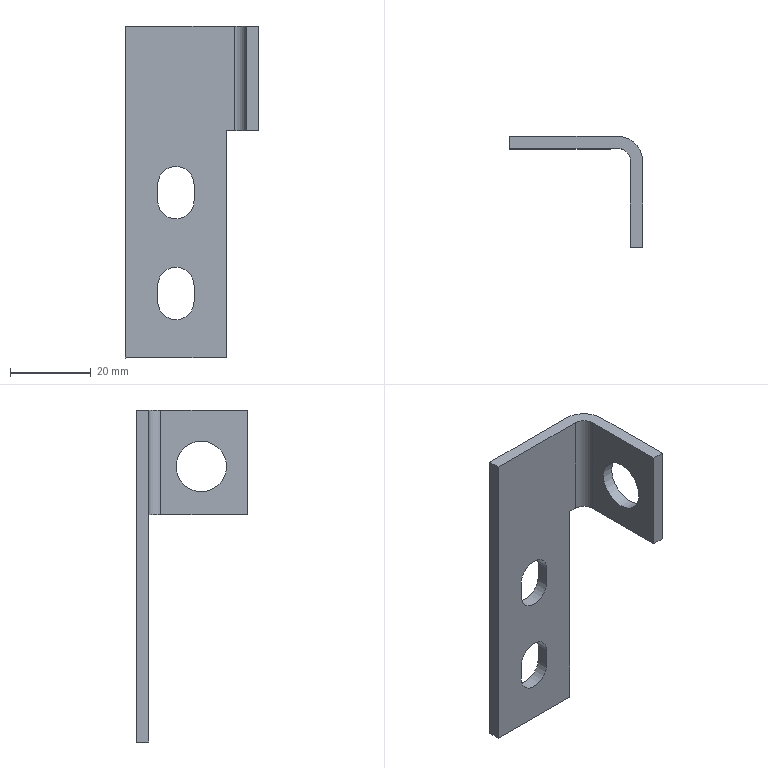Part | STEP file | lll_id850_x_t | 1 solid | 21 faces | box 33 x 27.5 x 82.328 mm | volume 7593 mm3 | plane 14 | cylinder 7 | commonest cylinder face diameters 9 x4 6 x1 12 x1 12.5 x1
STEP:
#1=CARTESIAN_POINT('',(3966.707,-571.677,70.922));
#2=VERTEX_POINT('',#1);
#3=CARTESIAN_POINT('',(3966.707,-571.677,153.25));
#4=VERTEX_POINT('',#3);
#5=CARTESIAN_POINT('',(3966.707,-571.677,181.75));
#6=DIRECTION('',(0.,0.,1.));
#7=VECTOR('',#6,1.);
#8=LINE('',#5,#7);
#9=EDGE_CURVE('',#2,#4,#8,.T.);
#10=ORIENTED_EDGE('',*,*,#9,.F.);
#11=CARTESIAN_POINT('',(3991.707,-571.677,70.922));
#12=VERTEX_POINT('',#11);
#13=CARTESIAN_POINT('',(4574.571,-571.677,70.922));
#14=DIRECTION('',(1.,0.,0.));
#15=VECTOR('',#14,1.);
#16=LINE('',#13,#15);
#17=EDGE_CURVE('',#2,#12,#16,.T.);
#18=ORIENTED_EDGE('',*,*,#17,.T.);
#19=CARTESIAN_POINT('',(3991.707,-571.677,127.25));
#20=VERTEX_POINT('',#19);
#21=CARTESIAN_POINT('',(3991.707,-571.677,176.75));
#22=DIRECTION('',(0.,0.,-1.));
#23=VECTOR('',#22,1.);
#24=LINE('',#21,#23);
#25=EDGE_CURVE('',#20,#12,#24,.T.);
#26=ORIENTED_EDGE('',*,*,#25,.F.);
#27=CARTESIAN_POINT('',(3993.707,-571.677,127.25));
#28=VERTEX_POINT('',#27);
#29=CARTESIAN_POINT('',(3964.707,-571.677,127.25));
#30=DIRECTION('',(1.,0.,0.));
#31=VECTOR('',#30,1.);
#32=LINE('',#29,#31);
#33=EDGE_CURVE('',#20,#28,#32,.T.);
#34=ORIENTED_EDGE('',*,*,#33,.T.);
#35=CARTESIAN_POINT('',(3993.707,-571.677,153.25));
#36=VERTEX_POINT('',#35);
#37=CARTESIAN_POINT('',(3993.707,-571.677,181.75));
#38=DIRECTION('',(0.,0.,1.));
#39=VECTOR('',#38,1.);
#40=LINE('',#37,#39);
#41=EDGE_CURVE('',#28,#36,#40,.T.);
#42=ORIENTED_EDGE('',*,*,#41,.T.);
#43=CARTESIAN_POINT('',(3964.707,-571.677,153.25));
#44=DIRECTION('',(1.,0.,0.));
#45=VECTOR('',#44,1.);
#46=LINE('',#43,#45);
#47=EDGE_CURVE('',#4,#36,#46,.T.);
#48=ORIENTED_EDGE('',*,*,#47,.F.);
#49=EDGE_LOOP('',(#10,#18,#26,#34,#42,#48));
#50=FACE_BOUND('',#49,.T.);
#51=CARTESIAN_POINT('',(3974.707,-571.677,84.922));
#52=VERTEX_POINT('',#51);
#53=CARTESIAN_POINT('',(3974.707,-571.677,88.922));
#54=VERTEX_POINT('',#53);
#55=CARTESIAN_POINT('',(3974.707,-571.677,23.922));
#56=DIRECTION('',(0.,0.,1.));
#57=VECTOR('',#56,1.);
#58=LINE('',#55,#57);
#59=EDGE_CURVE('',#52,#54,#58,.T.);
#60=ORIENTED_EDGE('',*,*,#59,.T.);
#61=CARTESIAN_POINT('',(3983.707,-571.677,88.922));
#62=VERTEX_POINT('',#61);
#63=CARTESIAN_POINT('',(3979.207,-571.677,88.922));
#64=DIRECTION('',(0.,1.,0.));
#65=DIRECTION('',(-1.,0.,0.));
#66=AXIS2_PLACEMENT_3D('',#63,#64,#65);
#67=CIRCLE('',#66,4.5);
#68=EDGE_CURVE('',#54,#62,#67,.T.);
#69=ORIENTED_EDGE('',*,*,#68,.T.);
#70=CARTESIAN_POINT('',(3983.707,-571.677,84.922));
#71=VERTEX_POINT('',#70);
#72=CARTESIAN_POINT('',(3983.707,-571.677,23.922));
#73=DIRECTION('',(0.,0.,-1.));
#74=VECTOR('',#73,1.);
#75=LINE('',#72,#74);
#76=EDGE_CURVE('',#62,#71,#75,.T.);
#77=ORIENTED_EDGE('',*,*,#76,.T.);
#78=CARTESIAN_POINT('',(3979.207,-571.677,84.922));
#79=DIRECTION('',(0.,1.,0.));
#80=DIRECTION('',(1.,0.,0.));
#81=AXIS2_PLACEMENT_3D('',#78,#79,#80);
#82=CIRCLE('',#81,4.5);
#83=EDGE_CURVE('',#71,#52,#82,.T.);
#84=ORIENTED_EDGE('',*,*,#83,.T.);
#85=EDGE_LOOP('',(#60,#69,#77,#84));
#86=FACE_BOUND('',#85,.T.);
#87=CARTESIAN_POINT('',(3974.707,-571.677,109.922));
#88=VERTEX_POINT('',#87);
#89=CARTESIAN_POINT('',(3974.707,-571.677,113.922));
#90=VERTEX_POINT('',#89);
#91=CARTESIAN_POINT('',(3974.707,-571.677,48.922));
#92=DIRECTION('',(0.,0.,1.));
#93=VECTOR('',#92,1.);
#94=LINE('',#91,#93);
#95=EDGE_CURVE('',#88,#90,#94,.T.);
#96=ORIENTED_EDGE('',*,*,#95,.T.);
#97=CARTESIAN_POINT('',(3983.707,-571.677,113.922));
#98=VERTEX_POINT('',#97);
#99=CARTESIAN_POINT('',(3979.207,-571.677,113.922));
#100=DIRECTION('',(0.,-1.,0.));
#101=DIRECTION('',(-1.,0.,0.));
#102=AXIS2_PLACEMENT_3D('',#99,#100,#101);
#103=CIRCLE('',#102,4.5);
#104=EDGE_CURVE('',#98,#90,#103,.T.);
#105=ORIENTED_EDGE('',*,*,#104,.F.);
#106=CARTESIAN_POINT('',(3983.707,-571.677,109.922));
#107=VERTEX_POINT('',#106);
#108=CARTESIAN_POINT('',(3983.707,-571.677,48.922));
#109=DIRECTION('',(0.,0.,-1.));
#110=VECTOR('',#109,1.);
#111=LINE('',#108,#110);
#112=EDGE_CURVE('',#98,#107,#111,.T.);
#113=ORIENTED_EDGE('',*,*,#112,.T.);
#114=CARTESIAN_POINT('',(3979.207,-571.677,109.922));
#115=DIRECTION('',(0.,1.,0.));
#116=DIRECTION('',(1.,0.,0.));
#117=AXIS2_PLACEMENT_3D('',#114,#115,#116);
#118=CIRCLE('',#117,4.5);
#119=EDGE_CURVE('',#107,#88,#118,.T.);
#120=ORIENTED_EDGE('',*,*,#119,.T.);
#121=EDGE_LOOP('',(#96,#105,#113,#120));
#122=FACE_BOUND('',#121,.T.);
#123=CARTESIAN_POINT('',(3964.707,-571.677,181.75));
#124=DIRECTION('',(0.,-1.,0.));
#125=DIRECTION('',(0.,0.,-1.));
#126=AXIS2_PLACEMENT_3D('',#123,#124,#125);
#127=PLANE('',#126);
#128=ADVANCED_FACE('',(#50,#86,#122),#127,.T.);
#129=CARTESIAN_POINT('',(3974.707,-568.677,88.922));
#130=VERTEX_POINT('',#129);
#131=CARTESIAN_POINT('',(3983.707,-568.677,88.922));
#132=VERTEX_POINT('',#131);
#133=CARTESIAN_POINT('',(3979.207,-568.677,88.922));
#134=DIRECTION('',(0.,1.,0.));
#135=DIRECTION('',(-1.,0.,0.));
#136=AXIS2_PLACEMENT_3D('',#133,#134,#135);
#137=CIRCLE('',#136,4.5);
#138=EDGE_CURVE('',#130,#132,#137,.T.);
#139=ORIENTED_EDGE('',*,*,#138,.F.);
#140=CARTESIAN_POINT('',(3974.707,-568.677,84.922));
#141=VERTEX_POINT('',#140);
#142=CARTESIAN_POINT('',(3974.707,-568.677,86.922));
#143=DIRECTION('',(0.,0.,1.));
#144=VECTOR('',#143,1.);
#145=LINE('',#142,#144);
#146=EDGE_CURVE('',#141,#130,#145,.T.);
#147=ORIENTED_EDGE('',*,*,#146,.F.);
#148=CARTESIAN_POINT('',(3983.707,-568.677,84.922));
#149=VERTEX_POINT('',#148);
#150=CARTESIAN_POINT('',(3979.207,-568.677,84.922));
#151=DIRECTION('',(0.,1.,0.));
#152=DIRECTION('',(-1.,0.,0.));
#153=AXIS2_PLACEMENT_3D('',#150,#151,#152);
#154=CIRCLE('',#153,4.5);
#155=EDGE_CURVE('',#149,#141,#154,.T.);
#156=ORIENTED_EDGE('',*,*,#155,.F.);
#157=CARTESIAN_POINT('',(3983.707,-568.677,86.922));
#158=DIRECTION('',(0.,0.,-1.));
#159=VECTOR('',#158,1.);
#160=LINE('',#157,#159);
#161=EDGE_CURVE('',#132,#149,#160,.T.);
#162=ORIENTED_EDGE('',*,*,#161,.F.);
#163=EDGE_LOOP('',(#139,#147,#156,#162));
#164=FACE_BOUND('',#163,.T.);
#165=CARTESIAN_POINT('',(3966.707,-568.677,70.922));
#166=VERTEX_POINT('',#165);
#167=CARTESIAN_POINT('',(3991.707,-568.677,70.922));
#168=VERTEX_POINT('',#167);
#169=CARTESIAN_POINT('',(4574.571,-568.677,70.922));
#170=DIRECTION('',(1.,0.,0.));
#171=VECTOR('',#170,1.);
#172=LINE('',#169,#171);
#173=EDGE_CURVE('',#166,#168,#172,.T.);
#174=ORIENTED_EDGE('',*,*,#173,.F.);
#175=CARTESIAN_POINT('',(3966.707,-568.677,153.25));
#176=VERTEX_POINT('',#175);
#177=CARTESIAN_POINT('',(3966.707,-568.677,-161.75));
#178=DIRECTION('',(0.,0.,1.));
#179=VECTOR('',#178,1.);
#180=LINE('',#177,#179);
#181=EDGE_CURVE('',#166,#176,#180,.T.);
#182=ORIENTED_EDGE('',*,*,#181,.T.);
#183=CARTESIAN_POINT('',(3993.707,-568.677,153.25));
#184=VERTEX_POINT('',#183);
#185=CARTESIAN_POINT('',(3908.841,-568.677,153.25));
#186=DIRECTION('',(1.,0.,0.));
#187=VECTOR('',#186,1.);
#188=LINE('',#185,#187);
#189=EDGE_CURVE('',#176,#184,#188,.T.);
#190=ORIENTED_EDGE('',*,*,#189,.T.);
#191=CARTESIAN_POINT('',(3993.707,-568.677,127.25));
#192=VERTEX_POINT('',#191);
#193=CARTESIAN_POINT('',(3993.707,-568.677,-161.75));
#194=DIRECTION('',(0.,0.,-1.));
#195=VECTOR('',#194,1.);
#196=LINE('',#193,#195);
#197=EDGE_CURVE('',#184,#192,#196,.T.);
#198=ORIENTED_EDGE('',*,*,#197,.T.);
#199=CARTESIAN_POINT('',(3991.707,-568.677,127.25));
#200=VERTEX_POINT('',#199);
#201=CARTESIAN_POINT('',(4574.571,-568.677,127.25));
#202=DIRECTION('',(-1.,0.,0.));
#203=VECTOR('',#202,1.);
#204=LINE('',#201,#203);
#205=EDGE_CURVE('',#192,#200,#204,.T.);
#206=ORIENTED_EDGE('',*,*,#205,.T.);
#207=CARTESIAN_POINT('',(3991.707,-568.677,-166.75));
#208=DIRECTION('',(0.,0.,1.));
#209=VECTOR('',#208,1.);
#210=LINE('',#207,#209);
#211=EDGE_CURVE('',#168,#200,#210,.T.);
#212=ORIENTED_EDGE('',*,*,#211,.F.);
#213=EDGE_LOOP('',(#174,#182,#190,#198,#206,#212));
#214=FACE_BOUND('',#213,.T.);
#215=CARTESIAN_POINT('',(3974.707,-568.677,109.922));
#216=VERTEX_POINT('',#215);
#217=CARTESIAN_POINT('',(3983.707,-568.677,109.922));
#218=VERTEX_POINT('',#217);
#219=CARTESIAN_POINT('',(3979.207,-568.677,109.922));
#220=DIRECTION('',(0.,-1.,0.));
#221=DIRECTION('',(-1.,0.,0.));
#222=AXIS2_PLACEMENT_3D('',#219,#220,#221);
#223=CIRCLE('',#222,4.5);
#224=EDGE_CURVE('',#216,#218,#223,.T.);
#225=ORIENTED_EDGE('',*,*,#224,.T.);
#226=CARTESIAN_POINT('',(3983.707,-568.677,113.922));
#227=VERTEX_POINT('',#226);
#228=CARTESIAN_POINT('',(3983.707,-568.677,111.922));
#229=DIRECTION('',(0.,0.,-1.));
#230=VECTOR('',#229,1.);
#231=LINE('',#228,#230);
#232=EDGE_CURVE('',#227,#218,#231,.T.);
#233=ORIENTED_EDGE('',*,*,#232,.F.);
#234=CARTESIAN_POINT('',(3974.707,-568.677,113.922));
#235=VERTEX_POINT('',#234);
#236=CARTESIAN_POINT('',(3979.207,-568.677,113.922));
#237=DIRECTION('',(0.,-1.,0.));
#238=DIRECTION('',(-1.,0.,0.));
#239=AXIS2_PLACEMENT_3D('',#236,#237,#238);
#240=CIRCLE('',#239,4.5);
#241=EDGE_CURVE('',#227,#235,#240,.T.);
#242=ORIENTED_EDGE('',*,*,#241,.T.);
#243=CARTESIAN_POINT('',(3974.707,-568.677,111.922));
#244=DIRECTION('',(0.,0.,1.));
#245=VECTOR('',#244,1.);
#246=LINE('',#243,#245);
#247=EDGE_CURVE('',#216,#235,#246,.T.);
#248=ORIENTED_EDGE('',*,*,#247,.F.);
#249=EDGE_LOOP('',(#225,#233,#242,#248));
#250=FACE_BOUND('',#249,.T.);
#251=CARTESIAN_POINT('',(4574.571,-568.677,-161.75));
#252=DIRECTION('',(0.,-1.,0.));
#253=DIRECTION('',(0.,0.,-1.));
#254=AXIS2_PLACEMENT_3D('',#251,#252,#253);
#255=PLANE('',#254);
#256=ADVANCED_FACE('',(#164,#214,#250),#255,.F.);
#257=CARTESIAN_POINT('',(3999.707,-584.727,145.5));
#258=VERTEX_POINT('',#257);
#259=CARTESIAN_POINT('',(3999.707,-584.727,139.25));
#260=DIRECTION('',(-1.,0.,0.));
#261=DIRECTION('',(0.,0.,1.));
#262=AXIS2_PLACEMENT_3D('',#259,#260,#261);
#263=CIRCLE('',#262,6.25);
#264=EDGE_CURVE('',#258,#258,#263,.T.);
#265=ORIENTED_EDGE('',*,*,#264,.F.);
#266=EDGE_LOOP('',(#265));
#267=FACE_BOUND('',#266,.T.);
#268=CARTESIAN_POINT('',(3996.707,-584.727,145.5));
#269=VERTEX_POINT('',#268);
#270=CARTESIAN_POINT('',(3996.707,-584.727,139.25));
#271=DIRECTION('',(-1.,0.,0.));
#272=DIRECTION('',(0.,0.,1.));
#273=AXIS2_PLACEMENT_3D('',#270,#271,#272);
#274=CIRCLE('',#273,6.25);
#275=EDGE_CURVE('',#269,#269,#274,.T.);
#276=ORIENTED_EDGE('',*,*,#275,.T.);
#277=EDGE_LOOP('',(#276));
#278=FACE_BOUND('',#277,.T.);
#279=CARTESIAN_POINT('',(4003.259,-584.727,139.25));
#280=DIRECTION('',(-1.,0.,0.));
#281=DIRECTION('',(0.,0.,-1.));
#282=AXIS2_PLACEMENT_3D('',#279,#280,#281);
#283=CYLINDRICAL_SURFACE('',#282,6.25);
#284=ADVANCED_FACE('',(#267,#278),#283,.F.);
#285=CARTESIAN_POINT('',(3999.707,-596.177,127.25));
#286=VERTEX_POINT('',#285);
#287=CARTESIAN_POINT('',(3999.707,-574.677,127.25));
#288=VERTEX_POINT('',#287);
#289=CARTESIAN_POINT('',(3999.707,-563.177,127.25));
#290=DIRECTION('',(0.,1.,0.));
#291=VECTOR('',#290,1.);
#292=LINE('',#289,#291);
#293=EDGE_CURVE('',#286,#288,#292,.T.);
#294=ORIENTED_EDGE('',*,*,#293,.T.);
#295=CARTESIAN_POINT('',(3999.707,-574.677,153.25));
#296=VERTEX_POINT('',#295);
#297=CARTESIAN_POINT('',(3999.707,-574.677,181.75));
#298=DIRECTION('',(0.,0.,1.));
#299=VECTOR('',#298,1.);
#300=LINE('',#297,#299);
#301=EDGE_CURVE('',#288,#296,#300,.T.);
#302=ORIENTED_EDGE('',*,*,#301,.T.);
#303=CARTESIAN_POINT('',(3999.707,-596.177,153.25));
#304=VERTEX_POINT('',#303);
#305=CARTESIAN_POINT('',(3999.707,-338.177,153.25));
#306=DIRECTION('',(0.,-1.,0.));
#307=VECTOR('',#306,1.);
#308=LINE('',#305,#307);
#309=EDGE_CURVE('',#296,#304,#308,.T.);
#310=ORIENTED_EDGE('',*,*,#309,.T.);
#311=CARTESIAN_POINT('',(3999.707,-596.177,181.75));
#312=DIRECTION('',(0.,0.,-1.));
#313=VECTOR('',#312,1.);
#314=LINE('',#311,#313);
#315=EDGE_CURVE('',#304,#286,#314,.T.);
#316=ORIENTED_EDGE('',*,*,#315,.T.);
#317=EDGE_LOOP('',(#294,#302,#310,#316));
#318=FACE_BOUND('',#317,.T.);
#319=ORIENTED_EDGE('',*,*,#264,.T.);
#320=EDGE_LOOP('',(#319));
#321=FACE_BOUND('',#320,.T.);
#322=CARTESIAN_POINT('',(3999.707,-563.177,181.75));
#323=DIRECTION('',(1.,0.,0.));
#324=DIRECTION('',(0.,0.,1.));
#325=AXIS2_PLACEMENT_3D('',#322,#323,#324);
#326=PLANE('',#325);
#327=ADVANCED_FACE('',(#318,#321),#326,.T.);
#328=CARTESIAN_POINT('',(3996.707,-596.177,153.25));
#329=VERTEX_POINT('',#328);
#330=CARTESIAN_POINT('',(3996.707,-596.177,127.25));
#331=VERTEX_POINT('',#330);
#332=CARTESIAN_POINT('',(3996.707,-596.177,164.25));
#333=DIRECTION('',(0.,0.,-1.));
#334=VECTOR('',#333,1.);
#335=LINE('',#332,#334);
#336=EDGE_CURVE('',#329,#331,#335,.T.);
#337=ORIENTED_EDGE('',*,*,#336,.T.);
#338=CARTESIAN_POINT('',(4011.057,-596.177,127.25));
#339=DIRECTION('',(1.,0.,0.));
#340=VECTOR('',#339,1.);
#341=LINE('',#338,#340);
#342=EDGE_CURVE('',#331,#286,#341,.T.);
#343=ORIENTED_EDGE('',*,*,#342,.T.);
#344=ORIENTED_EDGE('',*,*,#315,.F.);
#345=CARTESIAN_POINT('',(4011.057,-596.177,153.25));
#346=DIRECTION('',(1.,0.,0.));
#347=VECTOR('',#346,1.);
#348=LINE('',#345,#347);
#349=EDGE_CURVE('',#329,#304,#348,.T.);
#350=ORIENTED_EDGE('',*,*,#349,.F.);
#351=EDGE_LOOP('',(#337,#343,#344,#350));
#352=FACE_OUTER_BOUND('',#351,.T.);
#353=CARTESIAN_POINT('',(4011.057,-596.177,148.25));
#354=DIRECTION('',(0.,-1.,0.));
#355=DIRECTION('',(0.,0.,-1.));
#356=AXIS2_PLACEMENT_3D('',#353,#354,#355);
#357=PLANE('',#356);
#358=ADVANCED_FACE('',(#352),#357,.T.);
#359=CARTESIAN_POINT('',(3996.707,-574.677,153.25));
#360=VERTEX_POINT('',#359);
#361=CARTESIAN_POINT('',(3996.707,-338.177,153.25));
#362=DIRECTION('',(0.,-1.,0.));
#363=VECTOR('',#362,1.);
#364=LINE('',#361,#363);
#365=EDGE_CURVE('',#360,#329,#364,.T.);
#366=ORIENTED_EDGE('',*,*,#365,.F.);
#367=CARTESIAN_POINT('',(3996.707,-574.677,127.25));
#368=VERTEX_POINT('',#367);
#369=CARTESIAN_POINT('',(3996.707,-574.677,164.25));
#370=DIRECTION('',(0.,0.,-1.));
#371=VECTOR('',#370,1.);
#372=LINE('',#369,#371);
#373=EDGE_CURVE('',#360,#368,#372,.T.);
#374=ORIENTED_EDGE('',*,*,#373,.T.);
#375=CARTESIAN_POINT('',(3996.707,-564.677,127.25));
#376=DIRECTION('',(0.,1.,0.));
#377=VECTOR('',#376,1.);
#378=LINE('',#375,#377);
#379=EDGE_CURVE('',#331,#368,#378,.T.);
#380=ORIENTED_EDGE('',*,*,#379,.F.);
#381=ORIENTED_EDGE('',*,*,#336,.F.);
#382=EDGE_LOOP('',(#366,#374,#380,#381));
#383=FACE_BOUND('',#382,.T.);
#384=ORIENTED_EDGE('',*,*,#275,.F.);
#385=EDGE_LOOP('',(#384));
#386=FACE_BOUND('',#385,.T.);
#387=CARTESIAN_POINT('',(3996.707,-564.677,164.25));
#388=DIRECTION('',(1.,0.,0.));
#389=DIRECTION('',(0.,0.,1.));
#390=AXIS2_PLACEMENT_3D('',#387,#388,#389);
#391=PLANE('',#390);
#392=ADVANCED_FACE('',(#383,#386),#391,.F.);
#393=CARTESIAN_POINT('',(3993.707,-574.677,127.25));
#394=DIRECTION('',(0.,0.,1.));
#395=DIRECTION('',(-1.,0.,0.));
#396=AXIS2_PLACEMENT_3D('',#393,#394,#395);
#397=CIRCLE('',#396,3.);
#398=EDGE_CURVE('',#368,#28,#397,.T.);
#399=ORIENTED_EDGE('',*,*,#398,.F.);
#400=ORIENTED_EDGE('',*,*,#373,.F.);
#401=CARTESIAN_POINT('',(3993.707,-574.677,153.25));
#402=DIRECTION('',(0.,0.,-1.));
#403=DIRECTION('',(-1.,0.,0.));
#404=AXIS2_PLACEMENT_3D('',#401,#402,#403);
#405=CIRCLE('',#404,3.);
#406=EDGE_CURVE('',#36,#360,#405,.T.);
#407=ORIENTED_EDGE('',*,*,#406,.F.);
#408=ORIENTED_EDGE('',*,*,#41,.F.);
#409=EDGE_LOOP('',(#399,#400,#407,#408));
#410=FACE_OUTER_BOUND('',#409,.T.);
#411=CARTESIAN_POINT('',(3993.707,-574.677,181.75));
#412=DIRECTION('',(0.,0.,1.));
#413=DIRECTION('',(-1.,0.,0.));
#414=AXIS2_PLACEMENT_3D('',#411,#412,#413);
#415=CYLINDRICAL_SURFACE('',#414,3.);
#416=ADVANCED_FACE('',(#410),#415,.F.);
#417=ORIENTED_EDGE('',*,*,#189,.F.);
#418=CARTESIAN_POINT('',(3966.707,-338.177,153.25));
#419=DIRECTION('',(0.,1.,0.));
#420=VECTOR('',#419,1.);
#421=LINE('',#418,#420);
#422=EDGE_CURVE('',#4,#176,#421,.T.);
#423=ORIENTED_EDGE('',*,*,#422,.F.);
#424=ORIENTED_EDGE('',*,*,#47,.T.);
#425=ORIENTED_EDGE('',*,*,#406,.T.);
#426=ORIENTED_EDGE('',*,*,#365,.T.);
#427=ORIENTED_EDGE('',*,*,#349,.T.);
#428=ORIENTED_EDGE('',*,*,#309,.F.);
#429=CARTESIAN_POINT('',(3993.707,-574.677,153.25));
#430=DIRECTION('',(0.,0.,1.));
#431=DIRECTION('',(-1.,0.,0.));
#432=AXIS2_PLACEMENT_3D('',#429,#430,#431);
#433=CIRCLE('',#432,6.);
#434=EDGE_CURVE('',#296,#184,#433,.T.);
#435=ORIENTED_EDGE('',*,*,#434,.T.);
#436=EDGE_LOOP('',(#417,#423,#424,#425,#426,#427,#428,#435));
#437=FACE_OUTER_BOUND('',#436,.T.);
#438=CARTESIAN_POINT('',(3908.841,-338.177,153.25));
#439=DIRECTION('',(0.,0.,-1.));
#440=DIRECTION('',(1.,0.,0.));
#441=AXIS2_PLACEMENT_3D('',#438,#439,#440);
#442=PLANE('',#441);
#443=ADVANCED_FACE('',(#437),#442,.F.);
#444=ORIENTED_EDGE('',*,*,#434,.F.);
#445=ORIENTED_EDGE('',*,*,#301,.F.);
#446=CARTESIAN_POINT('',(3993.707,-574.677,127.25));
#447=DIRECTION('',(0.,0.,-1.));
#448=DIRECTION('',(-1.,0.,0.));
#449=AXIS2_PLACEMENT_3D('',#446,#447,#448);
#450=CIRCLE('',#449,6.);
#451=EDGE_CURVE('',#192,#288,#450,.T.);
#452=ORIENTED_EDGE('',*,*,#451,.F.);
#453=ORIENTED_EDGE('',*,*,#197,.F.);
#454=EDGE_LOOP('',(#444,#445,#452,#453));
#455=FACE_OUTER_BOUND('',#454,.T.);
#456=CARTESIAN_POINT('',(3993.707,-574.677,-161.75));
#457=DIRECTION('',(0.,0.,1.));
#458=DIRECTION('',(-1.,0.,0.));
#459=AXIS2_PLACEMENT_3D('',#456,#457,#458);
#460=CYLINDRICAL_SURFACE('',#459,6.);
#461=ADVANCED_FACE('',(#455),#460,.T.);
#462=CARTESIAN_POINT('',(3991.707,-495.177,127.25));
#463=DIRECTION('',(0.,1.,0.));
#464=VECTOR('',#463,1.);
#465=LINE('',#462,#464);
#466=EDGE_CURVE('',#20,#200,#465,.T.);
#467=ORIENTED_EDGE('',*,*,#466,.T.);
#468=ORIENTED_EDGE('',*,*,#205,.F.);
#469=ORIENTED_EDGE('',*,*,#451,.T.);
#470=ORIENTED_EDGE('',*,*,#293,.F.);
#471=ORIENTED_EDGE('',*,*,#342,.F.);
#472=ORIENTED_EDGE('',*,*,#379,.T.);
#473=ORIENTED_EDGE('',*,*,#398,.T.);
#474=ORIENTED_EDGE('',*,*,#33,.F.);
#475=EDGE_LOOP('',(#467,#468,#469,#470,#471,#472,#473,#474));
#476=FACE_OUTER_BOUND('',#475,.T.);
#477=CARTESIAN_POINT('',(4020.057,-495.177,127.25));
#478=DIRECTION('',(0.,0.,-1.));
#479=DIRECTION('',(-1.,0.,0.));
#480=AXIS2_PLACEMENT_3D('',#477,#478,#479);
#481=PLANE('',#480);
#482=ADVANCED_FACE('',(#476),#481,.T.);
#483=ORIENTED_EDGE('',*,*,#211,.T.);
#484=ORIENTED_EDGE('',*,*,#466,.F.);
#485=ORIENTED_EDGE('',*,*,#25,.T.);
#486=CARTESIAN_POINT('',(3991.707,-555.677,70.922));
#487=DIRECTION('',(0.,-1.,0.));
#488=VECTOR('',#487,1.);
#489=LINE('',#486,#488);
#490=EDGE_CURVE('',#168,#12,#489,.T.);
#491=ORIENTED_EDGE('',*,*,#490,.F.);
#492=EDGE_LOOP('',(#483,#484,#485,#491));
#493=FACE_OUTER_BOUND('',#492,.T.);
#494=CARTESIAN_POINT('',(3991.707,-555.677,123.25));
#495=DIRECTION('',(1.,0.,0.));
#496=DIRECTION('',(0.,0.,1.));
#497=AXIS2_PLACEMENT_3D('',#494,#495,#496);
#498=PLANE('',#497);
#499=ADVANCED_FACE('',(#493),#498,.T.);
#500=ORIENTED_EDGE('',*,*,#17,.F.);
#501=CARTESIAN_POINT('',(3966.707,-853.677,70.922));
#502=DIRECTION('',(0.,-1.,0.));
#503=VECTOR('',#502,1.);
#504=LINE('',#501,#503);
#505=EDGE_CURVE('',#166,#2,#504,.T.);
#506=ORIENTED_EDGE('',*,*,#505,.F.);
#507=ORIENTED_EDGE('',*,*,#173,.T.);
#508=ORIENTED_EDGE('',*,*,#490,.T.);
#509=EDGE_LOOP('',(#500,#506,#507,#508));
#510=FACE_OUTER_BOUND('',#509,.T.);
#511=CARTESIAN_POINT('',(4574.571,-853.677,70.922));
#512=DIRECTION('',(0.,0.,1.));
#513=DIRECTION('',(0.,-1.,0.));
#514=AXIS2_PLACEMENT_3D('',#511,#512,#513);
#515=PLANE('',#514);
#516=ADVANCED_FACE('',(#510),#515,.F.);
#517=CARTESIAN_POINT('',(3974.707,-1812.677,113.922));
#518=DIRECTION('',(0.,1.,0.));
#519=VECTOR('',#518,1.);
#520=LINE('',#517,#519);
#521=EDGE_CURVE('',#90,#235,#520,.T.);
#522=ORIENTED_EDGE('',*,*,#521,.T.);
#523=ORIENTED_EDGE('',*,*,#241,.F.);
#524=CARTESIAN_POINT('',(3983.707,-1812.677,113.922));
#525=DIRECTION('',(0.,-1.,0.));
#526=VECTOR('',#525,1.);
#527=LINE('',#524,#526);
#528=EDGE_CURVE('',#227,#98,#527,.T.);
#529=ORIENTED_EDGE('',*,*,#528,.T.);
#530=ORIENTED_EDGE('',*,*,#104,.T.);
#531=EDGE_LOOP('',(#522,#523,#529,#530));
#532=FACE_OUTER_BOUND('',#531,.T.);
#533=CARTESIAN_POINT('',(3979.207,-582.677,113.922));
#534=DIRECTION('',(0.,1.,0.));
#535=DIRECTION('',(1.,0.,0.));
#536=AXIS2_PLACEMENT_3D('',#533,#534,#535);
#537=CYLINDRICAL_SURFACE('',#536,4.5);
#538=ADVANCED_FACE('',(#532),#537,.F.);
#539=ORIENTED_EDGE('',*,*,#112,.F.);
#540=ORIENTED_EDGE('',*,*,#528,.F.);
#541=ORIENTED_EDGE('',*,*,#232,.T.);
#542=CARTESIAN_POINT('',(3983.707,-532.677,109.922));
#543=DIRECTION('',(0.,1.,0.));
#544=VECTOR('',#543,1.);
#545=LINE('',#542,#544);
#546=EDGE_CURVE('',#107,#218,#545,.T.);
#547=ORIENTED_EDGE('',*,*,#546,.F.);
#548=EDGE_LOOP('',(#539,#540,#541,#547));
#549=FACE_OUTER_BOUND('',#548,.T.);
#550=CARTESIAN_POINT('',(3983.707,-532.677,111.922));
#551=DIRECTION('',(1.,0.,0.));
#552=DIRECTION('',(0.,1.,0.));
#553=AXIS2_PLACEMENT_3D('',#550,#551,#552);
#554=PLANE('',#553);
#555=ADVANCED_FACE('',(#549),#554,.F.);
#556=ORIENTED_EDGE('',*,*,#119,.F.);
#557=ORIENTED_EDGE('',*,*,#546,.T.);
#558=ORIENTED_EDGE('',*,*,#224,.F.);
#559=CARTESIAN_POINT('',(3974.707,-532.677,109.922));
#560=DIRECTION('',(0.,1.,0.));
#561=VECTOR('',#560,1.);
#562=LINE('',#559,#561);
#563=EDGE_CURVE('',#88,#216,#562,.T.);
#564=ORIENTED_EDGE('',*,*,#563,.F.);
#565=EDGE_LOOP('',(#556,#557,#558,#564));
#566=FACE_OUTER_BOUND('',#565,.T.);
#567=CARTESIAN_POINT('',(3979.207,-1812.677,109.922));
#568=DIRECTION('',(0.,1.,0.));
#569=DIRECTION('',(-1.,0.,0.));
#570=AXIS2_PLACEMENT_3D('',#567,#568,#569);
#571=CYLINDRICAL_SURFACE('',#570,4.5);
#572=ADVANCED_FACE('',(#566),#571,.F.);
#573=ORIENTED_EDGE('',*,*,#95,.F.);
#574=ORIENTED_EDGE('',*,*,#563,.T.);
#575=ORIENTED_EDGE('',*,*,#247,.T.);
#576=ORIENTED_EDGE('',*,*,#521,.F.);
#577=EDGE_LOOP('',(#573,#574,#575,#576));
#578=FACE_OUTER_BOUND('',#577,.T.);
#579=CARTESIAN_POINT('',(3974.707,-532.677,111.922));
#580=DIRECTION('',(-1.,0.,0.));
#581=DIRECTION('',(0.,-1.,0.));
#582=AXIS2_PLACEMENT_3D('',#579,#580,#581);
#583=PLANE('',#582);
#584=ADVANCED_FACE('',(#578),#583,.F.);
#585=ORIENTED_EDGE('',*,*,#59,.F.);
#586=CARTESIAN_POINT('',(3974.707,-532.677,84.922));
#587=DIRECTION('',(0.,1.,0.));
#588=VECTOR('',#587,1.);
#589=LINE('',#586,#588);
#590=EDGE_CURVE('',#52,#141,#589,.T.);
#591=ORIENTED_EDGE('',*,*,#590,.T.);
#592=ORIENTED_EDGE('',*,*,#146,.T.);
#593=CARTESIAN_POINT('',(3974.707,-1812.677,88.922));
#594=DIRECTION('',(0.,1.,0.));
#595=VECTOR('',#594,1.);
#596=LINE('',#593,#595);
#597=EDGE_CURVE('',#54,#130,#596,.T.);
#598=ORIENTED_EDGE('',*,*,#597,.F.);
#599=EDGE_LOOP('',(#585,#591,#592,#598));
#600=FACE_OUTER_BOUND('',#599,.T.);
#601=CARTESIAN_POINT('',(3974.707,-532.677,86.922));
#602=DIRECTION('',(-1.,0.,0.));
#603=DIRECTION('',(0.,-1.,0.));
#604=AXIS2_PLACEMENT_3D('',#601,#602,#603);
#605=PLANE('',#604);
#606=ADVANCED_FACE('',(#600),#605,.F.);
#607=ORIENTED_EDGE('',*,*,#83,.F.);
#608=CARTESIAN_POINT('',(3983.707,-532.677,84.922));
#609=DIRECTION('',(0.,1.,0.));
#610=VECTOR('',#609,1.);
#611=LINE('',#608,#610);
#612=EDGE_CURVE('',#71,#149,#611,.T.);
#613=ORIENTED_EDGE('',*,*,#612,.T.);
#614=ORIENTED_EDGE('',*,*,#155,.T.);
#615=ORIENTED_EDGE('',*,*,#590,.F.);
#616=EDGE_LOOP('',(#607,#613,#614,#615));
#617=FACE_OUTER_BOUND('',#616,.T.);
#618=CARTESIAN_POINT('',(3979.207,-1812.677,84.922));
#619=DIRECTION('',(0.,1.,0.));
#620=DIRECTION('',(-1.,0.,0.));
#621=AXIS2_PLACEMENT_3D('',#618,#619,#620);
#622=CYLINDRICAL_SURFACE('',#621,4.5);
#623=ADVANCED_FACE('',(#617),#622,.F.);
#624=ORIENTED_EDGE('',*,*,#76,.F.);
#625=CARTESIAN_POINT('',(3983.707,-1812.677,88.922));
#626=DIRECTION('',(0.,-1.,0.));
#627=VECTOR('',#626,1.);
#628=LINE('',#625,#627);
#629=EDGE_CURVE('',#132,#62,#628,.T.);
#630=ORIENTED_EDGE('',*,*,#629,.F.);
#631=ORIENTED_EDGE('',*,*,#161,.T.);
#632=ORIENTED_EDGE('',*,*,#612,.F.);
#633=EDGE_LOOP('',(#624,#630,#631,#632));
#634=FACE_OUTER_BOUND('',#633,.T.);
#635=CARTESIAN_POINT('',(3983.707,-532.677,86.922));
#636=DIRECTION('',(1.,0.,0.));
#637=DIRECTION('',(0.,1.,0.));
#638=AXIS2_PLACEMENT_3D('',#635,#636,#637);
#639=PLANE('',#638);
#640=ADVANCED_FACE('',(#634),#639,.F.);
#641=ORIENTED_EDGE('',*,*,#597,.T.);
#642=ORIENTED_EDGE('',*,*,#138,.T.);
#643=ORIENTED_EDGE('',*,*,#629,.T.);
#644=ORIENTED_EDGE('',*,*,#68,.F.);
#645=EDGE_LOOP('',(#641,#642,#643,#644));
#646=FACE_OUTER_BOUND('',#645,.T.);
#647=CARTESIAN_POINT('',(3979.207,-582.677,88.922));
#648=DIRECTION('',(0.,1.,0.));
#649=DIRECTION('',(1.,0.,0.));
#650=AXIS2_PLACEMENT_3D('',#647,#648,#649);
#651=CYLINDRICAL_SURFACE('',#650,4.5);
#652=ADVANCED_FACE('',(#646),#651,.F.);
#653=ORIENTED_EDGE('',*,*,#181,.F.);
#654=ORIENTED_EDGE('',*,*,#505,.T.);
#655=ORIENTED_EDGE('',*,*,#9,.T.);
#656=ORIENTED_EDGE('',*,*,#422,.T.);
#657=EDGE_LOOP('',(#653,#654,#655,#656));
#658=FACE_OUTER_BOUND('',#657,.T.);
#659=CARTESIAN_POINT('',(3966.707,-570.177,99.086));
#660=DIRECTION('',(1.,0.,0.));
#661=DIRECTION('',(0.,0.,1.));
#662=AXIS2_PLACEMENT_3D('',#659,#660,#661);
#663=PLANE('',#662);
#664=ADVANCED_FACE('',(#658),#663,.F.);
#665=CLOSED_SHELL('',(#128,#256,#284,#327,#358,#392,#416,#443,#461,#482,#499,#516,#538,#555,#572,#584,#606,#623,#640,#652,#664));
#666=MANIFOLD_SOLID_BREP('',#665);
#667=(LENGTH_UNIT()NAMED_UNIT(*)SI_UNIT(.MILLI.,.METRE.));
#668=UNCERTAINTY_MEASURE_WITH_UNIT(LENGTH_MEASURE(0.00002),#667,'','');
#669=(NAMED_UNIT(*)PLANE_ANGLE_UNIT()SI_UNIT($,.RADIAN.));
#670=PLANE_ANGLE_MEASURE_WITH_UNIT(PLANE_ANGLE_MEASURE(0.01745),#669);
#671=DIMENSIONAL_EXPONENTS(0.,0.,0.,0.,0.,0.,0.);
#672=(CONVERSION_BASED_UNIT('DEGREE',#670)NAMED_UNIT(#671)PLANE_ANGLE_UNIT());
#673=(NAMED_UNIT(*)SI_UNIT($,.STERADIAN.)SOLID_ANGLE_UNIT());
#674=(GEOMETRIC_REPRESENTATION_CONTEXT(3)GLOBAL_UNCERTAINTY_ASSIGNED_CONTEXT((#668))GLOBAL_UNIT_ASSIGNED_CONTEXT((#667,#672,#673))REPRESENTATION_CONTEXT('',''));
#675=ADVANCED_BREP_SHAPE_REPRESENTATION('',(#666),#674);